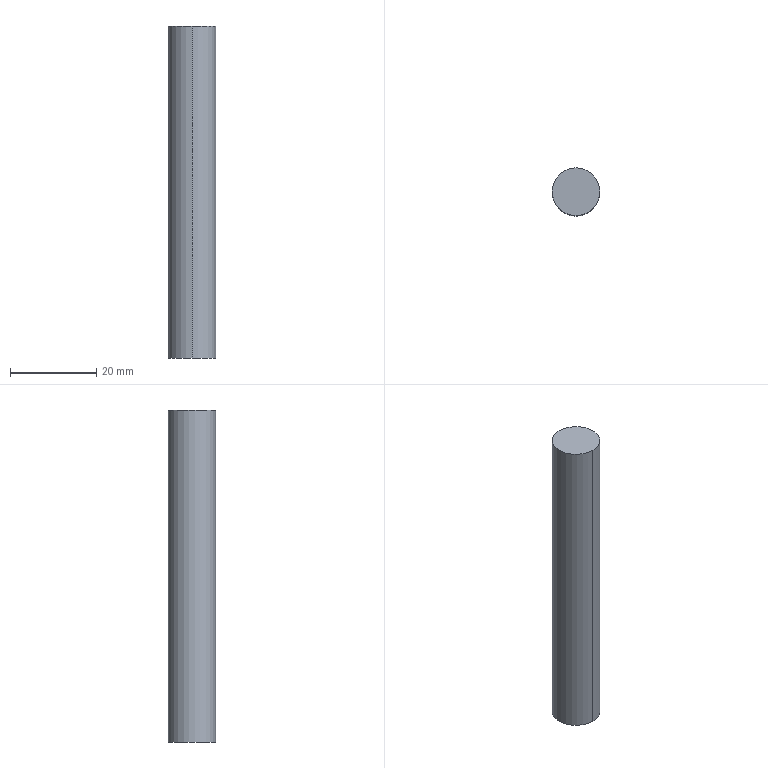Part | STEP file | 4-20.sldasm-Part-387 | 1 solid | 4 faces | box 11.11 x 11.11 x 77 mm | volume 7465 mm3 | cylinder 2 | plane 2 | commonest cylinder face diameters 11.11 x2
STEP:
#1=CARTESIAN_POINT('',(-50.,-405.555,154.));
#2=VERTEX_POINT('',#1);
#3=CARTESIAN_POINT('',(-50.,-394.445,154.));
#4=VERTEX_POINT('',#3);
#5=CARTESIAN_POINT('',(-50.,-400.,154.));
#6=DIRECTION('',(0.,0.,1.));
#7=DIRECTION('',(0.,-1.,0.));
#8=AXIS2_PLACEMENT_3D('',#5,#6,#7);
#9=CIRCLE('',#8,5.555);
#10=EDGE_CURVE('',#2,#4,#9,.T.);
#11=ORIENTED_EDGE('',*,*,#10,.T.);
#12=CARTESIAN_POINT('',(-50.,-394.445,231.));
#13=VERTEX_POINT('',#12);
#14=CARTESIAN_POINT('',(-50.,-394.445,129.));
#15=DIRECTION('',(0.,0.,1.));
#16=VECTOR('',#15,1000.);
#17=LINE('',#14,#16);
#18=EDGE_CURVE('',#4,#13,#17,.T.);
#19=ORIENTED_EDGE('',*,*,#18,.T.);
#20=CARTESIAN_POINT('',(-50.,-405.555,231.));
#21=VERTEX_POINT('',#20);
#22=CARTESIAN_POINT('',(-50.,-400.,231.));
#23=DIRECTION('',(0.,0.,1.));
#24=DIRECTION('',(1.,0.,0.));
#25=AXIS2_PLACEMENT_3D('',#22,#23,#24);
#26=CIRCLE('',#25,5.555);
#27=EDGE_CURVE('',#21,#13,#26,.T.);
#28=ORIENTED_EDGE('',*,*,#27,.F.);
#29=CARTESIAN_POINT('',(-50.,-405.555,129.));
#30=DIRECTION('',(0.,0.,1.));
#31=VECTOR('',#30,1000.);
#32=LINE('',#29,#31);
#33=EDGE_CURVE('',#2,#21,#32,.T.);
#34=ORIENTED_EDGE('',*,*,#33,.F.);
#35=EDGE_LOOP('',(#11,#19,#28,#34));
#36=FACE_OUTER_BOUND('',#35,.T.);
#37=CARTESIAN_POINT('',(-50.,-400.,129.));
#38=DIRECTION('',(0.,0.,1.));
#39=DIRECTION('',(0.,-1.,0.));
#40=AXIS2_PLACEMENT_3D('',#37,#38,#39);
#41=CYLINDRICAL_SURFACE('',#40,5.555);
#42=ADVANCED_FACE('',(#36),#41,.T.);
#43=ORIENTED_EDGE('',*,*,#18,.F.);
#44=CARTESIAN_POINT('',(-50.,-400.,154.));
#45=DIRECTION('',(0.,0.,1.));
#46=DIRECTION('',(0.,-1.,0.));
#47=AXIS2_PLACEMENT_3D('',#44,#45,#46);
#48=CIRCLE('',#47,5.555);
#49=EDGE_CURVE('',#4,#2,#48,.T.);
#50=ORIENTED_EDGE('',*,*,#49,.T.);
#51=ORIENTED_EDGE('',*,*,#33,.T.);
#52=CARTESIAN_POINT('',(-50.,-400.,231.));
#53=DIRECTION('',(0.,0.,1.));
#54=DIRECTION('',(1.,0.,0.));
#55=AXIS2_PLACEMENT_3D('',#52,#53,#54);
#56=CIRCLE('',#55,5.555);
#57=EDGE_CURVE('',#13,#21,#56,.T.);
#58=ORIENTED_EDGE('',*,*,#57,.F.);
#59=EDGE_LOOP('',(#43,#50,#51,#58));
#60=FACE_OUTER_BOUND('',#59,.T.);
#61=CARTESIAN_POINT('',(-50.,-400.,129.));
#62=DIRECTION('',(0.,0.,1.));
#63=DIRECTION('',(0.,-1.,0.));
#64=AXIS2_PLACEMENT_3D('',#61,#62,#63);
#65=CYLINDRICAL_SURFACE('',#64,5.555);
#66=ADVANCED_FACE('',(#60),#65,.T.);
#67=ORIENTED_EDGE('',*,*,#10,.F.);
#68=ORIENTED_EDGE('',*,*,#49,.F.);
#69=EDGE_LOOP('',(#67,#68));
#70=FACE_OUTER_BOUND('',#69,.T.);
#71=CARTESIAN_POINT('',(25.,-400.,154.));
#72=DIRECTION('',(0.,0.,1.));
#73=DIRECTION('',(0.,-1.,0.));
#74=AXIS2_PLACEMENT_3D('',#71,#72,#73);
#75=PLANE('',#74);
#76=ADVANCED_FACE('',(#70),#75,.F.);
#77=ORIENTED_EDGE('',*,*,#27,.T.);
#78=ORIENTED_EDGE('',*,*,#57,.T.);
#79=EDGE_LOOP('',(#77,#78));
#80=FACE_OUTER_BOUND('',#79,.T.);
#81=CARTESIAN_POINT('',(0.,420.,231.));
#82=DIRECTION('',(0.,0.,1.));
#83=DIRECTION('',(1.,0.,0.));
#84=AXIS2_PLACEMENT_3D('',#81,#82,#83);
#85=PLANE('',#84);
#86=ADVANCED_FACE('',(#80),#85,.T.);
#87=CLOSED_SHELL('',(#42,#66,#76,#86));
#88=MANIFOLD_SOLID_BREP('',#87);
#89=CARTESIAN_POINT('',(0.,0.,0.));
#90=DIRECTION('',(0.,0.,1.));
#91=DIRECTION('',(1.,0.,0.));
#92=AXIS2_PLACEMENT_3D('',#89,#90,#91);
#93=(LENGTH_UNIT()NAMED_UNIT(*)SI_UNIT(.MILLI.,.METRE.));
#94=UNCERTAINTY_MEASURE_WITH_UNIT(LENGTH_MEASURE(0.00001),#93,'','');
#95=(NAMED_UNIT(*)PLANE_ANGLE_UNIT()SI_UNIT($,.RADIAN.));
#96=(NAMED_UNIT(*)SI_UNIT($,.STERADIAN.)SOLID_ANGLE_UNIT());
#97=(GEOMETRIC_REPRESENTATION_CONTEXT(3)GLOBAL_UNCERTAINTY_ASSIGNED_CONTEXT((#94))GLOBAL_UNIT_ASSIGNED_CONTEXT((#93,#95,#96))REPRESENTATION_CONTEXT('',''));
#98=ADVANCED_BREP_SHAPE_REPRESENTATION('',(#88,#92),#97);